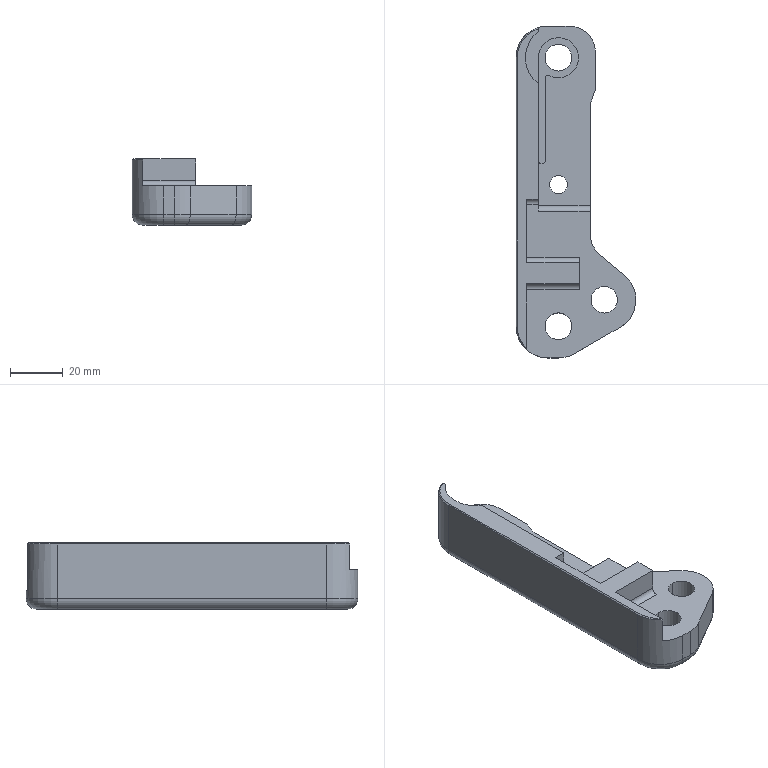Part | NX | features BREP 1 | 1 solid | 71 faces | box 45.321 x 125.509 x 25 mm | volume 49329 mm3 | cylinder 36 | plane 26 | torus 7 | cone 2 | commonest cylinder face diameters 8 x8 4 x4 10.1 x4 24 x4 2 x3 15.2 x3